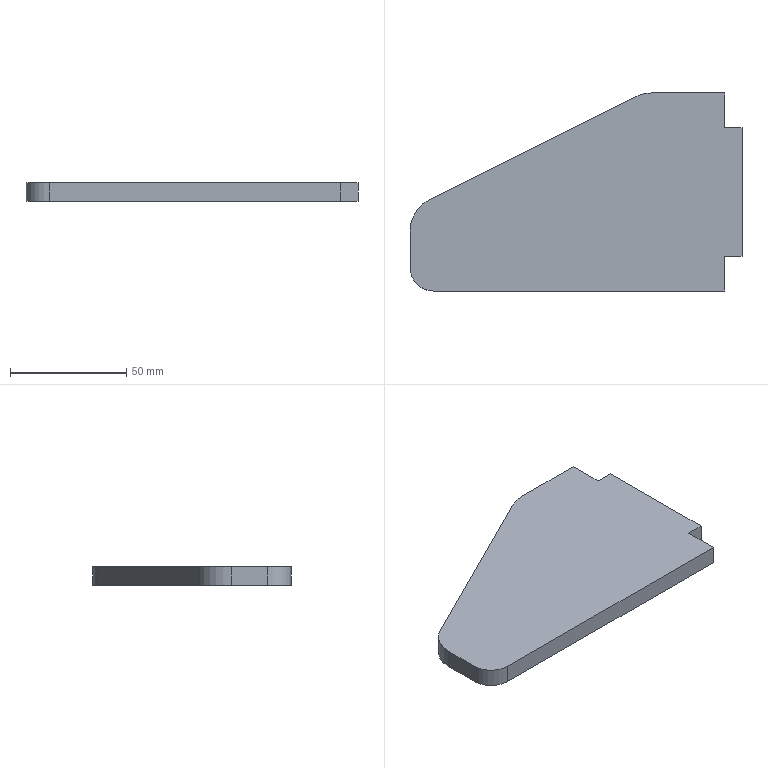Part | SolidWorks | features FlatPattern 1, SMBaseFlange 1, SheetMetal 1 | 1 solid | 14 faces | box 142.5 x 85 x 8 mm | volume 74805 mm3 | plane 11 | cylinder 3 | commonest cylinder face diameters 30 x2 20 x1
STEP:
#1=CARTESIAN_POINT('',(-1115.506,559.062,0.));
#2=VERTEX_POINT('',#1);
#3=CARTESIAN_POINT('',(-990.506,559.062,0.));
#4=VERTEX_POINT('',#3);
#5=CARTESIAN_POINT('',(-990.506,559.062,0.));
#6=DIRECTION('',(1.,0.,0.));
#7=VECTOR('',#6,1000.);
#8=LINE('',#5,#7);
#9=EDGE_CURVE('',#2,#4,#8,.T.);
#10=ORIENTED_EDGE('',*,*,#9,.F.);
#11=CARTESIAN_POINT('',(-1115.506,559.062,-8.));
#12=VERTEX_POINT('',#11);
#13=CARTESIAN_POINT('',(-1115.506,559.062,-8.));
#14=DIRECTION('',(0.,0.,1.));
#15=VECTOR('',#14,1000.);
#16=LINE('',#13,#15);
#17=EDGE_CURVE('',#12,#2,#16,.T.);
#18=ORIENTED_EDGE('',*,*,#17,.F.);
#19=CARTESIAN_POINT('',(-990.506,559.062,-8.));
#20=VERTEX_POINT('',#19);
#21=CARTESIAN_POINT('',(-990.506,559.062,-8.));
#22=DIRECTION('',(1.,0.,0.));
#23=VECTOR('',#22,1000.);
#24=LINE('',#21,#23);
#25=EDGE_CURVE('',#12,#20,#24,.T.);
#26=ORIENTED_EDGE('',*,*,#25,.T.);
#27=CARTESIAN_POINT('',(-990.506,559.062,-8.));
#28=DIRECTION('',(0.,0.,1.));
#29=VECTOR('',#28,1000.);
#30=LINE('',#27,#29);
#31=EDGE_CURVE('',#20,#4,#30,.T.);
#32=ORIENTED_EDGE('',*,*,#31,.T.);
#33=EDGE_LOOP('',(#10,#18,#26,#32));
#34=FACE_OUTER_BOUND('',#33,.T.);
#35=CARTESIAN_POINT('',(-990.506,559.062,-8.));
#36=DIRECTION('',(0.,-1.,0.));
#37=DIRECTION('',(1.,0.,0.));
#38=AXIS2_PLACEMENT_3D('',#35,#36,#37);
#39=PLANE('',#38);
#40=ADVANCED_FACE('',(#34),#39,.T.);
#41=CARTESIAN_POINT('',(-1125.506,569.062,0.));
#42=VERTEX_POINT('',#41);
#43=CARTESIAN_POINT('',(-1115.506,569.062,0.));
#44=DIRECTION('',(0.,0.,1.));
#45=DIRECTION('',(-1.,0.,0.));
#46=AXIS2_PLACEMENT_3D('',#43,#44,#45);
#47=CIRCLE('',#46,10.);
#48=EDGE_CURVE('',#42,#2,#47,.T.);
#49=ORIENTED_EDGE('',*,*,#48,.F.);
#50=CARTESIAN_POINT('',(-1125.506,569.062,-8.));
#51=VERTEX_POINT('',#50);
#52=CARTESIAN_POINT('',(-1125.506,569.062,-8.));
#53=DIRECTION('',(0.,0.,1.));
#54=VECTOR('',#53,1000.);
#55=LINE('',#52,#54);
#56=EDGE_CURVE('',#51,#42,#55,.T.);
#57=ORIENTED_EDGE('',*,*,#56,.F.);
#58=CARTESIAN_POINT('',(-1115.506,569.062,-8.));
#59=DIRECTION('',(0.,0.,1.));
#60=DIRECTION('',(-1.,0.,0.));
#61=AXIS2_PLACEMENT_3D('',#58,#59,#60);
#62=CIRCLE('',#61,10.);
#63=EDGE_CURVE('',#51,#12,#62,.T.);
#64=ORIENTED_EDGE('',*,*,#63,.T.);
#65=ORIENTED_EDGE('',*,*,#17,.T.);
#66=EDGE_LOOP('',(#49,#57,#64,#65));
#67=FACE_OUTER_BOUND('',#66,.T.);
#68=CARTESIAN_POINT('',(-1115.506,569.062,-8.));
#69=DIRECTION('',(0.,0.,1.));
#70=DIRECTION('',(1.,0.,0.));
#71=AXIS2_PLACEMENT_3D('',#68,#69,#70);
#72=CYLINDRICAL_SURFACE('',#71,10.);
#73=ADVANCED_FACE('',(#67),#72,.T.);
#74=CARTESIAN_POINT('',(-1125.506,584.791,0.));
#75=VERTEX_POINT('',#74);
#76=CARTESIAN_POINT('',(-1125.506,569.062,0.));
#77=DIRECTION('',(0.,-1.,0.));
#78=VECTOR('',#77,1000.);
#79=LINE('',#76,#78);
#80=EDGE_CURVE('',#75,#42,#79,.T.);
#81=ORIENTED_EDGE('',*,*,#80,.F.);
#82=CARTESIAN_POINT('',(-1125.506,584.791,-8.));
#83=VERTEX_POINT('',#82);
#84=CARTESIAN_POINT('',(-1125.506,584.791,-8.));
#85=DIRECTION('',(0.,0.,1.));
#86=VECTOR('',#85,1000.);
#87=LINE('',#84,#86);
#88=EDGE_CURVE('',#83,#75,#87,.T.);
#89=ORIENTED_EDGE('',*,*,#88,.F.);
#90=CARTESIAN_POINT('',(-1125.506,569.062,-8.));
#91=DIRECTION('',(0.,-1.,0.));
#92=VECTOR('',#91,1000.);
#93=LINE('',#90,#92);
#94=EDGE_CURVE('',#83,#51,#93,.T.);
#95=ORIENTED_EDGE('',*,*,#94,.T.);
#96=ORIENTED_EDGE('',*,*,#56,.T.);
#97=EDGE_LOOP('',(#81,#89,#95,#96));
#98=FACE_OUTER_BOUND('',#97,.T.);
#99=CARTESIAN_POINT('',(-1125.506,569.062,-8.));
#100=DIRECTION('',(-1.,0.,0.));
#101=DIRECTION('',(0.,0.,1.));
#102=AXIS2_PLACEMENT_3D('',#99,#100,#101);
#103=PLANE('',#102);
#104=ADVANCED_FACE('',(#98),#103,.T.);
#105=CARTESIAN_POINT('',(-1117.214,598.208,0.));
#106=VERTEX_POINT('',#105);
#107=CARTESIAN_POINT('',(-1110.506,584.791,0.));
#108=DIRECTION('',(0.,0.,1.));
#109=DIRECTION('',(-1.,0.,0.));
#110=AXIS2_PLACEMENT_3D('',#107,#108,#109);
#111=CIRCLE('',#110,15.);
#112=EDGE_CURVE('',#106,#75,#111,.T.);
#113=ORIENTED_EDGE('',*,*,#112,.F.);
#114=CARTESIAN_POINT('',(-1117.214,598.208,-8.));
#115=VERTEX_POINT('',#114);
#116=CARTESIAN_POINT('',(-1117.214,598.208,-8.));
#117=DIRECTION('',(0.,0.,1.));
#118=VECTOR('',#117,1000.);
#119=LINE('',#116,#118);
#120=EDGE_CURVE('',#115,#106,#119,.T.);
#121=ORIENTED_EDGE('',*,*,#120,.F.);
#122=CARTESIAN_POINT('',(-1110.506,584.791,-8.));
#123=DIRECTION('',(0.,0.,1.));
#124=DIRECTION('',(-1.,0.,0.));
#125=AXIS2_PLACEMENT_3D('',#122,#123,#124);
#126=CIRCLE('',#125,15.);
#127=EDGE_CURVE('',#115,#83,#126,.T.);
#128=ORIENTED_EDGE('',*,*,#127,.T.);
#129=ORIENTED_EDGE('',*,*,#88,.T.);
#130=EDGE_LOOP('',(#113,#121,#128,#129));
#131=FACE_OUTER_BOUND('',#130,.T.);
#132=CARTESIAN_POINT('',(-1110.506,584.791,-8.));
#133=DIRECTION('',(0.,0.,1.));
#134=DIRECTION('',(1.,0.,0.));
#135=AXIS2_PLACEMENT_3D('',#132,#133,#134);
#136=CYLINDRICAL_SURFACE('',#135,15.);
#137=ADVANCED_FACE('',(#131),#136,.T.);
#138=CARTESIAN_POINT('',(-1028.673,642.478,0.));
#139=VERTEX_POINT('',#138);
#140=CARTESIAN_POINT('',(-1117.214,598.208,0.));
#141=DIRECTION('',(-0.8944,-0.4472,0.));
#142=VECTOR('',#141,1000.);
#143=LINE('',#140,#142);
#144=EDGE_CURVE('',#139,#106,#143,.T.);
#145=ORIENTED_EDGE('',*,*,#144,.F.);
#146=CARTESIAN_POINT('',(-1028.673,642.478,-8.));
#147=VERTEX_POINT('',#146);
#148=CARTESIAN_POINT('',(-1028.673,642.478,-8.));
#149=DIRECTION('',(0.,0.,1.));
#150=VECTOR('',#149,1000.);
#151=LINE('',#148,#150);
#152=EDGE_CURVE('',#147,#139,#151,.T.);
#153=ORIENTED_EDGE('',*,*,#152,.F.);
#154=CARTESIAN_POINT('',(-1117.214,598.208,-8.));
#155=DIRECTION('',(-0.8944,-0.4472,0.));
#156=VECTOR('',#155,1000.);
#157=LINE('',#154,#156);
#158=EDGE_CURVE('',#147,#115,#157,.T.);
#159=ORIENTED_EDGE('',*,*,#158,.T.);
#160=ORIENTED_EDGE('',*,*,#120,.T.);
#161=EDGE_LOOP('',(#145,#153,#159,#160));
#162=FACE_OUTER_BOUND('',#161,.T.);
#163=CARTESIAN_POINT('',(-1117.214,598.208,-8.));
#164=DIRECTION('',(-0.4472,0.8944,0.));
#165=DIRECTION('',(-0.8944,-0.4472,0.));
#166=AXIS2_PLACEMENT_3D('',#163,#164,#165);
#167=PLANE('',#166);
#168=ADVANCED_FACE('',(#162),#167,.T.);
#169=CARTESIAN_POINT('',(-1021.965,644.062,0.));
#170=VERTEX_POINT('',#169);
#171=CARTESIAN_POINT('',(-1021.965,629.062,0.));
#172=DIRECTION('',(0.,0.,1.));
#173=DIRECTION('',(-1.,0.,0.));
#174=AXIS2_PLACEMENT_3D('',#171,#172,#173);
#175=CIRCLE('',#174,15.);
#176=EDGE_CURVE('',#170,#139,#175,.T.);
#177=ORIENTED_EDGE('',*,*,#176,.F.);
#178=CARTESIAN_POINT('',(-1021.965,644.062,-8.));
#179=VERTEX_POINT('',#178);
#180=CARTESIAN_POINT('',(-1021.965,644.062,-8.));
#181=DIRECTION('',(0.,0.,1.));
#182=VECTOR('',#181,1000.);
#183=LINE('',#180,#182);
#184=EDGE_CURVE('',#179,#170,#183,.T.);
#185=ORIENTED_EDGE('',*,*,#184,.F.);
#186=CARTESIAN_POINT('',(-1021.965,629.062,-8.));
#187=DIRECTION('',(0.,0.,1.));
#188=DIRECTION('',(-1.,0.,0.));
#189=AXIS2_PLACEMENT_3D('',#186,#187,#188);
#190=CIRCLE('',#189,15.);
#191=EDGE_CURVE('',#179,#147,#190,.T.);
#192=ORIENTED_EDGE('',*,*,#191,.T.);
#193=ORIENTED_EDGE('',*,*,#152,.T.);
#194=EDGE_LOOP('',(#177,#185,#192,#193));
#195=FACE_OUTER_BOUND('',#194,.T.);
#196=CARTESIAN_POINT('',(-1021.965,629.062,-8.));
#197=DIRECTION('',(0.,0.,1.));
#198=DIRECTION('',(1.,0.,0.));
#199=AXIS2_PLACEMENT_3D('',#196,#197,#198);
#200=CYLINDRICAL_SURFACE('',#199,15.);
#201=ADVANCED_FACE('',(#195),#200,.T.);
#202=CARTESIAN_POINT('',(-990.506,644.062,0.));
#203=VERTEX_POINT('',#202);
#204=CARTESIAN_POINT('',(-1021.965,644.062,0.));
#205=DIRECTION('',(-1.,0.,0.));
#206=VECTOR('',#205,1000.);
#207=LINE('',#204,#206);
#208=EDGE_CURVE('',#203,#170,#207,.T.);
#209=ORIENTED_EDGE('',*,*,#208,.F.);
#210=CARTESIAN_POINT('',(-990.506,644.062,-8.));
#211=VERTEX_POINT('',#210);
#212=CARTESIAN_POINT('',(-990.506,644.062,-8.));
#213=DIRECTION('',(0.,0.,1.));
#214=VECTOR('',#213,1000.);
#215=LINE('',#212,#214);
#216=EDGE_CURVE('',#211,#203,#215,.T.);
#217=ORIENTED_EDGE('',*,*,#216,.F.);
#218=CARTESIAN_POINT('',(-1021.965,644.062,-8.));
#219=DIRECTION('',(-1.,0.,0.));
#220=VECTOR('',#219,1000.);
#221=LINE('',#218,#220);
#222=EDGE_CURVE('',#211,#179,#221,.T.);
#223=ORIENTED_EDGE('',*,*,#222,.T.);
#224=ORIENTED_EDGE('',*,*,#184,.T.);
#225=EDGE_LOOP('',(#209,#217,#223,#224));
#226=FACE_OUTER_BOUND('',#225,.T.);
#227=CARTESIAN_POINT('',(-1021.965,644.062,-8.));
#228=DIRECTION('',(0.,1.,0.));
#229=DIRECTION('',(-1.,0.,0.));
#230=AXIS2_PLACEMENT_3D('',#227,#228,#229);
#231=PLANE('',#230);
#232=ADVANCED_FACE('',(#226),#231,.T.);
#233=CARTESIAN_POINT('',(-990.506,629.062,0.));
#234=VERTEX_POINT('',#233);
#235=CARTESIAN_POINT('',(-990.506,629.062,0.));
#236=DIRECTION('',(0.,1.,0.));
#237=VECTOR('',#236,1000.);
#238=LINE('',#235,#237);
#239=EDGE_CURVE('',#234,#203,#238,.T.);
#240=ORIENTED_EDGE('',*,*,#239,.F.);
#241=CARTESIAN_POINT('',(-990.506,629.062,-8.));
#242=VERTEX_POINT('',#241);
#243=CARTESIAN_POINT('',(-990.506,629.062,-8.));
#244=DIRECTION('',(0.,0.,1.));
#245=VECTOR('',#244,1000.);
#246=LINE('',#243,#245);
#247=EDGE_CURVE('',#242,#234,#246,.T.);
#248=ORIENTED_EDGE('',*,*,#247,.F.);
#249=CARTESIAN_POINT('',(-990.506,629.062,-8.));
#250=DIRECTION('',(0.,1.,0.));
#251=VECTOR('',#250,1000.);
#252=LINE('',#249,#251);
#253=EDGE_CURVE('',#242,#211,#252,.T.);
#254=ORIENTED_EDGE('',*,*,#253,.T.);
#255=ORIENTED_EDGE('',*,*,#216,.T.);
#256=EDGE_LOOP('',(#240,#248,#254,#255));
#257=FACE_OUTER_BOUND('',#256,.T.);
#258=CARTESIAN_POINT('',(-990.506,629.062,-8.));
#259=DIRECTION('',(1.,0.,0.));
#260=DIRECTION('',(0.,0.,-1.));
#261=AXIS2_PLACEMENT_3D('',#258,#259,#260);
#262=PLANE('',#261);
#263=ADVANCED_FACE('',(#257),#262,.T.);
#264=CARTESIAN_POINT('',(-983.006,629.062,0.));
#265=VERTEX_POINT('',#264);
#266=CARTESIAN_POINT('',(-983.006,629.062,0.));
#267=DIRECTION('',(-1.,0.,0.));
#268=VECTOR('',#267,1000.);
#269=LINE('',#266,#268);
#270=EDGE_CURVE('',#265,#234,#269,.T.);
#271=ORIENTED_EDGE('',*,*,#270,.F.);
#272=CARTESIAN_POINT('',(-983.006,629.062,-8.));
#273=VERTEX_POINT('',#272);
#274=CARTESIAN_POINT('',(-983.006,629.062,-8.));
#275=DIRECTION('',(0.,0.,1.));
#276=VECTOR('',#275,1000.);
#277=LINE('',#274,#276);
#278=EDGE_CURVE('',#273,#265,#277,.T.);
#279=ORIENTED_EDGE('',*,*,#278,.F.);
#280=CARTESIAN_POINT('',(-983.006,629.062,-8.));
#281=DIRECTION('',(-1.,0.,0.));
#282=VECTOR('',#281,1000.);
#283=LINE('',#280,#282);
#284=EDGE_CURVE('',#273,#242,#283,.T.);
#285=ORIENTED_EDGE('',*,*,#284,.T.);
#286=ORIENTED_EDGE('',*,*,#247,.T.);
#287=EDGE_LOOP('',(#271,#279,#285,#286));
#288=FACE_OUTER_BOUND('',#287,.T.);
#289=CARTESIAN_POINT('',(-983.006,629.062,-8.));
#290=DIRECTION('',(0.,1.,0.));
#291=DIRECTION('',(0.,0.,1.));
#292=AXIS2_PLACEMENT_3D('',#289,#290,#291);
#293=PLANE('',#292);
#294=ADVANCED_FACE('',(#288),#293,.T.);
#295=CARTESIAN_POINT('',(-983.006,574.062,0.));
#296=VERTEX_POINT('',#295);
#297=CARTESIAN_POINT('',(-983.006,574.062,0.));
#298=DIRECTION('',(0.,1.,0.));
#299=VECTOR('',#298,1000.);
#300=LINE('',#297,#299);
#301=EDGE_CURVE('',#296,#265,#300,.T.);
#302=ORIENTED_EDGE('',*,*,#301,.F.);
#303=CARTESIAN_POINT('',(-983.006,574.062,-8.));
#304=VERTEX_POINT('',#303);
#305=CARTESIAN_POINT('',(-983.006,574.062,-8.));
#306=DIRECTION('',(0.,0.,1.));
#307=VECTOR('',#306,1000.);
#308=LINE('',#305,#307);
#309=EDGE_CURVE('',#304,#296,#308,.T.);
#310=ORIENTED_EDGE('',*,*,#309,.F.);
#311=CARTESIAN_POINT('',(-983.006,574.062,-8.));
#312=DIRECTION('',(0.,1.,0.));
#313=VECTOR('',#312,1000.);
#314=LINE('',#311,#313);
#315=EDGE_CURVE('',#304,#273,#314,.T.);
#316=ORIENTED_EDGE('',*,*,#315,.T.);
#317=ORIENTED_EDGE('',*,*,#278,.T.);
#318=EDGE_LOOP('',(#302,#310,#316,#317));
#319=FACE_OUTER_BOUND('',#318,.T.);
#320=CARTESIAN_POINT('',(-983.006,574.062,-8.));
#321=DIRECTION('',(1.,0.,0.));
#322=DIRECTION('',(0.,0.,-1.));
#323=AXIS2_PLACEMENT_3D('',#320,#321,#322);
#324=PLANE('',#323);
#325=ADVANCED_FACE('',(#319),#324,.T.);
#326=CARTESIAN_POINT('',(-990.506,574.062,0.));
#327=VERTEX_POINT('',#326);
#328=CARTESIAN_POINT('',(-990.506,574.062,0.));
#329=DIRECTION('',(1.,0.,0.));
#330=VECTOR('',#329,1000.);
#331=LINE('',#328,#330);
#332=EDGE_CURVE('',#327,#296,#331,.T.);
#333=ORIENTED_EDGE('',*,*,#332,.F.);
#334=CARTESIAN_POINT('',(-990.506,574.062,-8.));
#335=VERTEX_POINT('',#334);
#336=CARTESIAN_POINT('',(-990.506,574.062,-8.));
#337=DIRECTION('',(0.,0.,1.));
#338=VECTOR('',#337,1000.);
#339=LINE('',#336,#338);
#340=EDGE_CURVE('',#335,#327,#339,.T.);
#341=ORIENTED_EDGE('',*,*,#340,.F.);
#342=CARTESIAN_POINT('',(-990.506,574.062,-8.));
#343=DIRECTION('',(1.,0.,0.));
#344=VECTOR('',#343,1000.);
#345=LINE('',#342,#344);
#346=EDGE_CURVE('',#335,#304,#345,.T.);
#347=ORIENTED_EDGE('',*,*,#346,.T.);
#348=ORIENTED_EDGE('',*,*,#309,.T.);
#349=EDGE_LOOP('',(#333,#341,#347,#348));
#350=FACE_OUTER_BOUND('',#349,.T.);
#351=CARTESIAN_POINT('',(-990.506,574.062,-8.));
#352=DIRECTION('',(0.,-1.,0.));
#353=DIRECTION('',(0.,0.,-1.));
#354=AXIS2_PLACEMENT_3D('',#351,#352,#353);
#355=PLANE('',#354);
#356=ADVANCED_FACE('',(#350),#355,.T.);
#357=CARTESIAN_POINT('',(-990.506,559.062,0.));
#358=DIRECTION('',(0.,1.,0.));
#359=VECTOR('',#358,1000.);
#360=LINE('',#357,#359);
#361=EDGE_CURVE('',#4,#327,#360,.T.);
#362=ORIENTED_EDGE('',*,*,#361,.F.);
#363=ORIENTED_EDGE('',*,*,#31,.F.);
#364=CARTESIAN_POINT('',(-990.506,559.062,-8.));
#365=DIRECTION('',(0.,1.,0.));
#366=VECTOR('',#365,1000.);
#367=LINE('',#364,#366);
#368=EDGE_CURVE('',#20,#335,#367,.T.);
#369=ORIENTED_EDGE('',*,*,#368,.T.);
#370=ORIENTED_EDGE('',*,*,#340,.T.);
#371=EDGE_LOOP('',(#362,#363,#369,#370));
#372=FACE_OUTER_BOUND('',#371,.T.);
#373=CARTESIAN_POINT('',(-990.506,559.062,-8.));
#374=DIRECTION('',(1.,0.,0.));
#375=DIRECTION('',(0.,0.,-1.));
#376=AXIS2_PLACEMENT_3D('',#373,#374,#375);
#377=PLANE('',#376);
#378=ADVANCED_FACE('',(#372),#377,.T.);
#379=ORIENTED_EDGE('',*,*,#25,.F.);
#380=ORIENTED_EDGE('',*,*,#63,.F.);
#381=ORIENTED_EDGE('',*,*,#94,.F.);
#382=ORIENTED_EDGE('',*,*,#127,.F.);
#383=ORIENTED_EDGE('',*,*,#158,.F.);
#384=ORIENTED_EDGE('',*,*,#191,.F.);
#385=ORIENTED_EDGE('',*,*,#222,.F.);
#386=ORIENTED_EDGE('',*,*,#253,.F.);
#387=ORIENTED_EDGE('',*,*,#284,.F.);
#388=ORIENTED_EDGE('',*,*,#315,.F.);
#389=ORIENTED_EDGE('',*,*,#346,.F.);
#390=ORIENTED_EDGE('',*,*,#368,.F.);
#391=EDGE_LOOP('',(#379,#380,#381,#382,#383,#384,#385,#386,#387,#388,#389,#390));
#392=FACE_OUTER_BOUND('',#391,.T.);
#393=CARTESIAN_POINT('',(-1115.506,569.062,-8.));
#394=DIRECTION('',(0.,0.,-1.));
#395=DIRECTION('',(-1.,0.,0.));
#396=AXIS2_PLACEMENT_3D('',#393,#394,#395);
#397=PLANE('',#396);
#398=ADVANCED_FACE('',(#392),#397,.T.);
#399=ORIENTED_EDGE('',*,*,#9,.T.);
#400=ORIENTED_EDGE('',*,*,#361,.T.);
#401=ORIENTED_EDGE('',*,*,#332,.T.);
#402=ORIENTED_EDGE('',*,*,#301,.T.);
#403=ORIENTED_EDGE('',*,*,#270,.T.);
#404=ORIENTED_EDGE('',*,*,#239,.T.);
#405=ORIENTED_EDGE('',*,*,#208,.T.);
#406=ORIENTED_EDGE('',*,*,#176,.T.);
#407=ORIENTED_EDGE('',*,*,#144,.T.);
#408=ORIENTED_EDGE('',*,*,#112,.T.);
#409=ORIENTED_EDGE('',*,*,#80,.T.);
#410=ORIENTED_EDGE('',*,*,#48,.T.);
#411=EDGE_LOOP('',(#399,#400,#401,#402,#403,#404,#405,#406,#407,#408,#409,#410));
#412=FACE_OUTER_BOUND('',#411,.T.);
#413=CARTESIAN_POINT('',(-1115.506,569.062,0.));
#414=DIRECTION('',(0.,0.,-1.));
#415=DIRECTION('',(-1.,0.,0.));
#416=AXIS2_PLACEMENT_3D('',#413,#414,#415);
#417=PLANE('',#416);
#418=ADVANCED_FACE('',(#412),#417,.F.);
#419=CLOSED_SHELL('',(#40,#73,#104,#137,#168,#201,#232,#263,#294,#325,#356,#378,#398,#418));
#420=MANIFOLD_SOLID_BREP('',#419);
#421=CARTESIAN_POINT('',(0.,0.,0.));
#422=DIRECTION('',(0.,0.,1.));
#423=DIRECTION('',(1.,0.,0.));
#424=AXIS2_PLACEMENT_3D('',#421,#422,#423);
#425=(LENGTH_UNIT()NAMED_UNIT(*)SI_UNIT(.MILLI.,.METRE.));
#426=UNCERTAINTY_MEASURE_WITH_UNIT(LENGTH_MEASURE(0.00001),#425,'','');
#427=(NAMED_UNIT(*)PLANE_ANGLE_UNIT()SI_UNIT($,.RADIAN.));
#428=(NAMED_UNIT(*)SI_UNIT($,.STERADIAN.)SOLID_ANGLE_UNIT());
#429=(GEOMETRIC_REPRESENTATION_CONTEXT(3)GLOBAL_UNCERTAINTY_ASSIGNED_CONTEXT((#426))GLOBAL_UNIT_ASSIGNED_CONTEXT((#425,#427,#428))REPRESENTATION_CONTEXT('',''));
#430=ADVANCED_BREP_SHAPE_REPRESENTATION('',(#420,#424),#429);